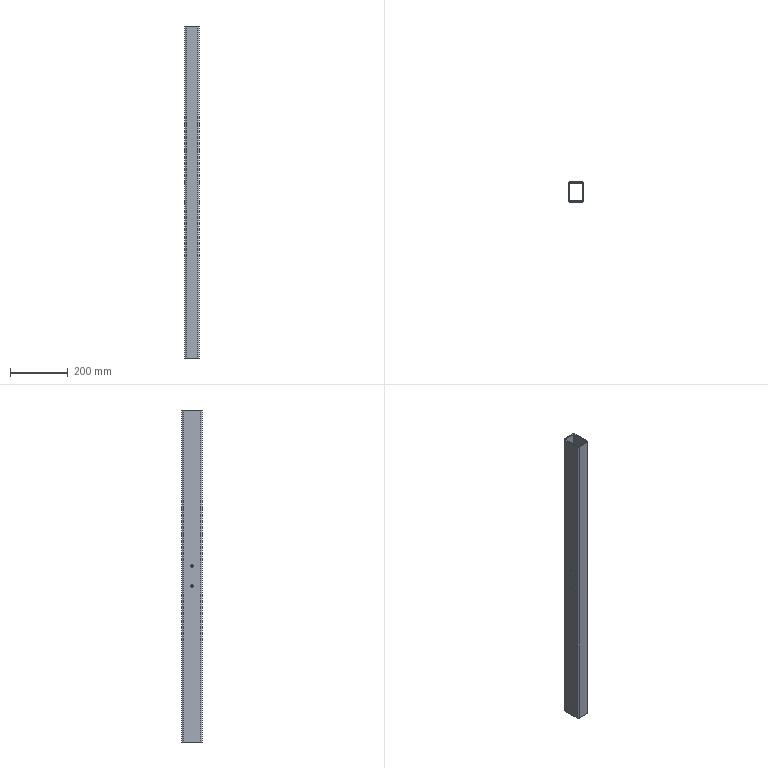Part | STEP file | Square steel 50×70×1150 | 1 solid | 26 faces | box 50 x 70 x 1150 mm | volume 1005690 mm3 | cylinder 16 | plane 10 | commonest cylinder face diameters 9 x8 2 x4 10 x4